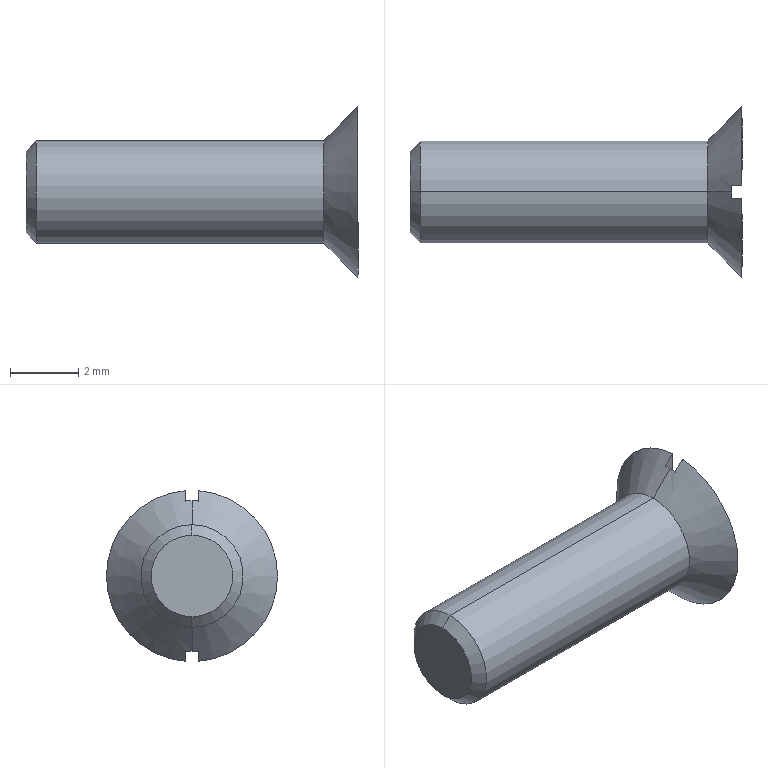Part | SolidWorks | features BaseBody 1 | 1 solid | 12 faces | box 9.7 x 5 x 4.984 mm | volume 73.349 mm3 | plane 6 | cone 4 | cylinder 2 | commonest cylinder face diameters 3 x2
STEP:
#1=CARTESIAN_POINT('',(30.,-10.25,11.75));
#2=VERTEX_POINT('',#1);
#3=CARTESIAN_POINT('',(30.,-10.25,8.75));
#4=VERTEX_POINT('',#3);
#5=CARTESIAN_POINT('',(30.,-10.25,10.25));
#6=DIRECTION('',(-1.,0.,0.));
#7=DIRECTION('',(0.,0.,1.));
#8=AXIS2_PLACEMENT_3D('',#5,#6,#7);
#9=CIRCLE('',#8,1.5);
#10=EDGE_CURVE('',#2,#4,#9,.T.);
#11=ORIENTED_EDGE('',*,*,#10,.T.);
#12=CARTESIAN_POINT('',(21.607,-10.25,8.75));
#13=VERTEX_POINT('',#12);
#14=CARTESIAN_POINT('',(25.803,-10.25,8.75));
#15=DIRECTION('',(-1.,0.,0.));
#16=VECTOR('',#15,1000.);
#17=LINE('',#14,#16);
#18=EDGE_CURVE('',#4,#13,#17,.T.);
#19=ORIENTED_EDGE('',*,*,#18,.T.);
#20=CARTESIAN_POINT('',(21.607,-10.25,11.75));
#21=VERTEX_POINT('',#20);
#22=CARTESIAN_POINT('',(21.607,-10.25,10.25));
#23=DIRECTION('',(1.,0.,0.));
#24=DIRECTION('',(0.,0.,1.));
#25=AXIS2_PLACEMENT_3D('',#22,#23,#24);
#26=CIRCLE('',#25,1.5);
#27=EDGE_CURVE('',#13,#21,#26,.T.);
#28=ORIENTED_EDGE('',*,*,#27,.T.);
#29=CARTESIAN_POINT('',(25.803,-10.25,11.75));
#30=DIRECTION('',(-1.,0.,0.));
#31=VECTOR('',#30,1000.);
#32=LINE('',#29,#31);
#33=EDGE_CURVE('',#2,#21,#32,.T.);
#34=ORIENTED_EDGE('',*,*,#33,.F.);
#35=EDGE_LOOP('',(#11,#19,#28,#34));
#36=FACE_OUTER_BOUND('',#35,.T.);
#37=CARTESIAN_POINT('',(25.803,-10.25,10.25));
#38=DIRECTION('',(-1.,0.,0.));
#39=DIRECTION('',(0.,0.,1.));
#40=AXIS2_PLACEMENT_3D('',#37,#38,#39);
#41=CYLINDRICAL_SURFACE('',#40,1.5);
#42=ADVANCED_FACE('',(#36),#41,.T.);
#43=ORIENTED_EDGE('',*,*,#10,.F.);
#44=CARTESIAN_POINT('',(30.7,-10.25,12.45));
#45=VERTEX_POINT('',#44);
#46=CARTESIAN_POINT('',(31.,-10.25,12.75));
#47=DIRECTION('',(0.7071,0.,0.7071));
#48=VECTOR('',#47,1000.);
#49=LINE('',#46,#48);
#50=EDGE_CURVE('',#2,#45,#49,.T.);
#51=ORIENTED_EDGE('',*,*,#50,.T.);
#52=CARTESIAN_POINT('',(30.7,-10.05,12.441));
#53=VERTEX_POINT('',#52);
#54=CARTESIAN_POINT('',(30.7,-10.25,10.25));
#55=DIRECTION('',(1.,0.,0.));
#56=DIRECTION('',(0.,0.,-1.));
#57=AXIS2_PLACEMENT_3D('',#54,#55,#56);
#58=CIRCLE('',#57,2.2);
#59=EDGE_CURVE('',#53,#45,#58,.T.);
#60=ORIENTED_EDGE('',*,*,#59,.F.);
#61=CARTESIAN_POINT('',(31.,-10.05,12.742));
#62=VERTEX_POINT('',#61);
#63=CARTESIAN_POINT('',(30.7,-10.05,12.441));
#64=CARTESIAN_POINT('',(30.8,-10.05,12.541));
#65=CARTESIAN_POINT('',(30.9,-10.05,12.642));
#66=CARTESIAN_POINT('',(31.,-10.05,12.742));
#67=B_SPLINE_CURVE_WITH_KNOTS('',3,(#63,#64,#65,#66),.UNSPECIFIED.,.F.,.F.,(4,4),(0.,0.000425),.UNSPECIFIED.);
#68=EDGE_CURVE('',#53,#62,#67,.T.);
#69=ORIENTED_EDGE('',*,*,#68,.T.);
#70=CARTESIAN_POINT('',(31.,-10.05,7.758));
#71=VERTEX_POINT('',#70);
#72=CARTESIAN_POINT('',(31.,-10.25,10.25));
#73=DIRECTION('',(-1.,0.,0.));
#74=DIRECTION('',(0.,0.,-1.));
#75=AXIS2_PLACEMENT_3D('',#72,#73,#74);
#76=CIRCLE('',#75,2.5);
#77=EDGE_CURVE('',#62,#71,#76,.T.);
#78=ORIENTED_EDGE('',*,*,#77,.T.);
#79=CARTESIAN_POINT('',(30.7,-10.05,8.059));
#80=VERTEX_POINT('',#79);
#81=CARTESIAN_POINT('',(31.,-10.05,7.758));
#82=CARTESIAN_POINT('',(30.9,-10.05,7.858));
#83=CARTESIAN_POINT('',(30.8,-10.05,7.959));
#84=CARTESIAN_POINT('',(30.7,-10.05,8.059));
#85=B_SPLINE_CURVE_WITH_KNOTS('',3,(#81,#82,#83,#84),.UNSPECIFIED.,.F.,.F.,(4,4),(0.,0.000425),.UNSPECIFIED.);
#86=EDGE_CURVE('',#71,#80,#85,.T.);
#87=ORIENTED_EDGE('',*,*,#86,.T.);
#88=CARTESIAN_POINT('',(30.7,-10.25,8.05));
#89=VERTEX_POINT('',#88);
#90=CARTESIAN_POINT('',(30.7,-10.25,10.25));
#91=DIRECTION('',(1.,0.,0.));
#92=DIRECTION('',(0.,0.,-1.));
#93=AXIS2_PLACEMENT_3D('',#90,#91,#92);
#94=CIRCLE('',#93,2.2);
#95=EDGE_CURVE('',#89,#80,#94,.T.);
#96=ORIENTED_EDGE('',*,*,#95,.F.);
#97=CARTESIAN_POINT('',(31.,-10.25,7.75));
#98=DIRECTION('',(0.7071,0.,-0.7071));
#99=VECTOR('',#98,1000.);
#100=LINE('',#97,#99);
#101=EDGE_CURVE('',#4,#89,#100,.T.);
#102=ORIENTED_EDGE('',*,*,#101,.F.);
#103=EDGE_LOOP('',(#43,#51,#60,#69,#78,#87,#96,#102));
#104=FACE_OUTER_BOUND('',#103,.T.);
#105=CARTESIAN_POINT('',(31.,-10.25,10.25));
#106=DIRECTION('',(1.,0.,0.));
#107=DIRECTION('',(0.,0.,-1.));
#108=AXIS2_PLACEMENT_3D('',#105,#106,#107);
#109=CONICAL_SURFACE('',#108,2.5,0.7854);
#110=ADVANCED_FACE('',(#104),#109,.T.);
#111=CARTESIAN_POINT('',(21.3,-10.25,9.057));
#112=VERTEX_POINT('',#111);
#113=CARTESIAN_POINT('',(21.3,-10.25,11.443));
#114=VERTEX_POINT('',#113);
#115=CARTESIAN_POINT('',(21.3,-10.25,10.25));
#116=DIRECTION('',(1.,0.,0.));
#117=DIRECTION('',(0.,0.,-1.));
#118=AXIS2_PLACEMENT_3D('',#115,#116,#117);
#119=CIRCLE('',#118,1.193);
#120=EDGE_CURVE('',#112,#114,#119,.T.);
#121=ORIENTED_EDGE('',*,*,#120,.T.);
#122=CARTESIAN_POINT('',(21.607,-10.25,11.75));
#123=DIRECTION('',(0.7071,0.,0.7071));
#124=VECTOR('',#123,1000.);
#125=LINE('',#122,#124);
#126=EDGE_CURVE('',#114,#21,#125,.T.);
#127=ORIENTED_EDGE('',*,*,#126,.T.);
#128=ORIENTED_EDGE('',*,*,#27,.F.);
#129=CARTESIAN_POINT('',(21.607,-10.25,8.75));
#130=DIRECTION('',(0.7071,0.,-0.7071));
#131=VECTOR('',#130,1000.);
#132=LINE('',#129,#131);
#133=EDGE_CURVE('',#112,#13,#132,.T.);
#134=ORIENTED_EDGE('',*,*,#133,.F.);
#135=EDGE_LOOP('',(#121,#127,#128,#134));
#136=FACE_OUTER_BOUND('',#135,.T.);
#137=CARTESIAN_POINT('',(21.607,-10.25,10.25));
#138=DIRECTION('',(1.,0.,0.));
#139=DIRECTION('',(0.,0.,-1.));
#140=AXIS2_PLACEMENT_3D('',#137,#138,#139);
#141=CONICAL_SURFACE('',#140,1.5,0.7854);
#142=ADVANCED_FACE('',(#136),#141,.T.);
#143=CARTESIAN_POINT('',(30.7,-10.45,12.441));
#144=VERTEX_POINT('',#143);
#145=CARTESIAN_POINT('',(30.7,-10.45,8.059));
#146=VERTEX_POINT('',#145);
#147=CARTESIAN_POINT('',(30.7,-10.45,12.75));
#148=DIRECTION('',(0.,0.,-1.));
#149=VECTOR('',#148,1000.);
#150=LINE('',#147,#149);
#151=EDGE_CURVE('',#144,#146,#150,.T.);
#152=ORIENTED_EDGE('',*,*,#151,.T.);
#153=CARTESIAN_POINT('',(30.7,-10.25,10.25));
#154=DIRECTION('',(1.,0.,0.));
#155=DIRECTION('',(0.,0.,-1.));
#156=AXIS2_PLACEMENT_3D('',#153,#154,#155);
#157=CIRCLE('',#156,2.2);
#158=EDGE_CURVE('',#146,#89,#157,.T.);
#159=ORIENTED_EDGE('',*,*,#158,.T.);
#160=ORIENTED_EDGE('',*,*,#95,.T.);
#161=CARTESIAN_POINT('',(30.7,-10.05,7.75));
#162=DIRECTION('',(0.,0.,1.));
#163=VECTOR('',#162,1000.);
#164=LINE('',#161,#163);
#165=EDGE_CURVE('',#80,#53,#164,.T.);
#166=ORIENTED_EDGE('',*,*,#165,.T.);
#167=ORIENTED_EDGE('',*,*,#59,.T.);
#168=CARTESIAN_POINT('',(30.7,-10.25,10.25));
#169=DIRECTION('',(1.,0.,0.));
#170=DIRECTION('',(0.,0.,-1.));
#171=AXIS2_PLACEMENT_3D('',#168,#169,#170);
#172=CIRCLE('',#171,2.2);
#173=EDGE_CURVE('',#45,#144,#172,.T.);
#174=ORIENTED_EDGE('',*,*,#173,.T.);
#175=EDGE_LOOP('',(#152,#159,#160,#166,#167,#174));
#176=FACE_OUTER_BOUND('',#175,.T.);
#177=CARTESIAN_POINT('',(30.7,-10.25,10.25));
#178=DIRECTION('',(1.,0.,0.));
#179=DIRECTION('',(0.,1.,0.));
#180=AXIS2_PLACEMENT_3D('',#177,#178,#179);
#181=PLANE('',#180);
#182=ADVANCED_FACE('',(#176),#181,.T.);
#183=CARTESIAN_POINT('',(31.,-10.45,7.758));
#184=VERTEX_POINT('',#183);
#185=CARTESIAN_POINT('',(31.,-10.45,12.742));
#186=VERTEX_POINT('',#185);
#187=CARTESIAN_POINT('',(31.,-10.45,10.25));
#188=DIRECTION('',(0.,0.,1.));
#189=VECTOR('',#188,1000.);
#190=LINE('',#187,#189);
#191=EDGE_CURVE('',#184,#186,#190,.T.);
#192=ORIENTED_EDGE('',*,*,#191,.F.);
#193=CARTESIAN_POINT('',(30.7,-10.45,8.059));
#194=CARTESIAN_POINT('',(30.8,-10.45,7.959));
#195=CARTESIAN_POINT('',(30.9,-10.45,7.858));
#196=CARTESIAN_POINT('',(31.,-10.45,7.758));
#197=B_SPLINE_CURVE_WITH_KNOTS('',3,(#193,#194,#195,#196),.UNSPECIFIED.,.F.,.F.,(4,4),(0.,0.000425),.UNSPECIFIED.);
#198=EDGE_CURVE('',#146,#184,#197,.T.);
#199=ORIENTED_EDGE('',*,*,#198,.F.);
#200=ORIENTED_EDGE('',*,*,#151,.F.);
#201=CARTESIAN_POINT('',(31.,-10.45,12.742));
#202=CARTESIAN_POINT('',(30.9,-10.45,12.642));
#203=CARTESIAN_POINT('',(30.8,-10.45,12.541));
#204=CARTESIAN_POINT('',(30.7,-10.45,12.441));
#205=B_SPLINE_CURVE_WITH_KNOTS('',3,(#201,#202,#203,#204),.UNSPECIFIED.,.F.,.F.,(4,4),(0.,0.000425),.UNSPECIFIED.);
#206=EDGE_CURVE('',#186,#144,#205,.T.);
#207=ORIENTED_EDGE('',*,*,#206,.F.);
#208=EDGE_LOOP('',(#192,#199,#200,#207));
#209=FACE_OUTER_BOUND('',#208,.T.);
#210=CARTESIAN_POINT('',(31.,-10.45,12.75));
#211=DIRECTION('',(0.,-1.,0.));
#212=DIRECTION('',(0.,0.,-1.));
#213=AXIS2_PLACEMENT_3D('',#210,#211,#212);
#214=PLANE('',#213);
#215=ADVANCED_FACE('',(#209),#214,.F.);
#216=ORIENTED_EDGE('',*,*,#165,.F.);
#217=ORIENTED_EDGE('',*,*,#86,.F.);
#218=CARTESIAN_POINT('',(31.,-10.05,10.25));
#219=DIRECTION('',(0.,0.,-1.));
#220=VECTOR('',#219,1000.);
#221=LINE('',#218,#220);
#222=EDGE_CURVE('',#62,#71,#221,.T.);
#223=ORIENTED_EDGE('',*,*,#222,.F.);
#224=ORIENTED_EDGE('',*,*,#68,.F.);
#225=EDGE_LOOP('',(#216,#217,#223,#224));
#226=FACE_OUTER_BOUND('',#225,.T.);
#227=CARTESIAN_POINT('',(31.,-10.05,7.75));
#228=DIRECTION('',(0.,1.,0.));
#229=DIRECTION('',(1.,0.,0.));
#230=AXIS2_PLACEMENT_3D('',#227,#228,#229);
#231=PLANE('',#230);
#232=ADVANCED_FACE('',(#226),#231,.F.);
#233=ORIENTED_EDGE('',*,*,#120,.F.);
#234=CARTESIAN_POINT('',(21.3,-10.25,10.25));
#235=DIRECTION('',(1.,0.,0.));
#236=DIRECTION('',(0.,0.,-1.));
#237=AXIS2_PLACEMENT_3D('',#234,#235,#236);
#238=CIRCLE('',#237,1.193);
#239=EDGE_CURVE('',#114,#112,#238,.T.);
#240=ORIENTED_EDGE('',*,*,#239,.F.);
#241=EDGE_LOOP('',(#233,#240));
#242=FACE_OUTER_BOUND('',#241,.T.);
#243=CARTESIAN_POINT('',(21.3,-9.653,10.25));
#244=DIRECTION('',(-1.,0.,0.));
#245=DIRECTION('',(0.,0.,1.));
#246=AXIS2_PLACEMENT_3D('',#243,#244,#245);
#247=PLANE('',#246);
#248=ADVANCED_FACE('',(#242),#247,.T.);
#249=CARTESIAN_POINT('',(31.,-10.25,10.25));
#250=DIRECTION('',(-1.,0.,0.));
#251=DIRECTION('',(0.,0.,-1.));
#252=AXIS2_PLACEMENT_3D('',#249,#250,#251);
#253=CIRCLE('',#252,2.5);
#254=EDGE_CURVE('',#184,#186,#253,.T.);
#255=ORIENTED_EDGE('',*,*,#254,.F.);
#256=ORIENTED_EDGE('',*,*,#191,.T.);
#257=EDGE_LOOP('',(#255,#256));
#258=FACE_OUTER_BOUND('',#257,.T.);
#259=CARTESIAN_POINT('',(31.,-9.,10.25));
#260=DIRECTION('',(1.,0.,0.));
#261=DIRECTION('',(0.,1.,0.));
#262=AXIS2_PLACEMENT_3D('',#259,#260,#261);
#263=PLANE('',#262);
#264=ADVANCED_FACE('',(#258),#263,.T.);
#265=ORIENTED_EDGE('',*,*,#222,.T.);
#266=ORIENTED_EDGE('',*,*,#77,.F.);
#267=EDGE_LOOP('',(#265,#266));
#268=FACE_OUTER_BOUND('',#267,.T.);
#269=CARTESIAN_POINT('',(31.,-9.,10.25));
#270=DIRECTION('',(1.,0.,0.));
#271=DIRECTION('',(0.,1.,0.));
#272=AXIS2_PLACEMENT_3D('',#269,#270,#271);
#273=PLANE('',#272);
#274=ADVANCED_FACE('',(#268),#273,.T.);
#275=ORIENTED_EDGE('',*,*,#126,.F.);
#276=ORIENTED_EDGE('',*,*,#239,.T.);
#277=ORIENTED_EDGE('',*,*,#133,.T.);
#278=CARTESIAN_POINT('',(21.607,-10.25,10.25));
#279=DIRECTION('',(1.,0.,0.));
#280=DIRECTION('',(0.,0.,1.));
#281=AXIS2_PLACEMENT_3D('',#278,#279,#280);
#282=CIRCLE('',#281,1.5);
#283=EDGE_CURVE('',#21,#13,#282,.T.);
#284=ORIENTED_EDGE('',*,*,#283,.F.);
#285=EDGE_LOOP('',(#275,#276,#277,#284));
#286=FACE_OUTER_BOUND('',#285,.T.);
#287=CARTESIAN_POINT('',(21.607,-10.25,10.25));
#288=DIRECTION('',(1.,0.,0.));
#289=DIRECTION('',(0.,0.,-1.));
#290=AXIS2_PLACEMENT_3D('',#287,#288,#289);
#291=CONICAL_SURFACE('',#290,1.5,0.7854);
#292=ADVANCED_FACE('',(#286),#291,.T.);
#293=ORIENTED_EDGE('',*,*,#50,.F.);
#294=CARTESIAN_POINT('',(30.,-10.25,10.25));
#295=DIRECTION('',(-1.,0.,0.));
#296=DIRECTION('',(0.,0.,1.));
#297=AXIS2_PLACEMENT_3D('',#294,#295,#296);
#298=CIRCLE('',#297,1.5);
#299=EDGE_CURVE('',#4,#2,#298,.T.);
#300=ORIENTED_EDGE('',*,*,#299,.F.);
#301=ORIENTED_EDGE('',*,*,#101,.T.);
#302=ORIENTED_EDGE('',*,*,#158,.F.);
#303=ORIENTED_EDGE('',*,*,#198,.T.);
#304=ORIENTED_EDGE('',*,*,#254,.T.);
#305=ORIENTED_EDGE('',*,*,#206,.T.);
#306=ORIENTED_EDGE('',*,*,#173,.F.);
#307=EDGE_LOOP('',(#293,#300,#301,#302,#303,#304,#305,#306));
#308=FACE_OUTER_BOUND('',#307,.T.);
#309=CARTESIAN_POINT('',(31.,-10.25,10.25));
#310=DIRECTION('',(1.,0.,0.));
#311=DIRECTION('',(0.,0.,-1.));
#312=AXIS2_PLACEMENT_3D('',#309,#310,#311);
#313=CONICAL_SURFACE('',#312,2.5,0.7854);
#314=ADVANCED_FACE('',(#308),#313,.T.);
#315=ORIENTED_EDGE('',*,*,#18,.F.);
#316=ORIENTED_EDGE('',*,*,#299,.T.);
#317=ORIENTED_EDGE('',*,*,#33,.T.);
#318=ORIENTED_EDGE('',*,*,#283,.T.);
#319=EDGE_LOOP('',(#315,#316,#317,#318));
#320=FACE_OUTER_BOUND('',#319,.T.);
#321=CARTESIAN_POINT('',(25.803,-10.25,10.25));
#322=DIRECTION('',(-1.,0.,0.));
#323=DIRECTION('',(0.,0.,1.));
#324=AXIS2_PLACEMENT_3D('',#321,#322,#323);
#325=CYLINDRICAL_SURFACE('',#324,1.5);
#326=ADVANCED_FACE('',(#320),#325,.T.);
#327=CLOSED_SHELL('',(#42,#110,#142,#182,#215,#232,#248,#264,#274,#292,#314,#326));
#328=MANIFOLD_SOLID_BREP('',#327);
#329=CARTESIAN_POINT('',(0.,0.,0.));
#330=DIRECTION('',(0.,0.,1.));
#331=DIRECTION('',(1.,0.,0.));
#332=AXIS2_PLACEMENT_3D('',#329,#330,#331);
#333=(LENGTH_UNIT()NAMED_UNIT(*)SI_UNIT(.MILLI.,.METRE.));
#334=UNCERTAINTY_MEASURE_WITH_UNIT(LENGTH_MEASURE(0.00001),#333,'','');
#335=(NAMED_UNIT(*)PLANE_ANGLE_UNIT()SI_UNIT($,.RADIAN.));
#336=(NAMED_UNIT(*)SI_UNIT($,.STERADIAN.)SOLID_ANGLE_UNIT());
#337=(GEOMETRIC_REPRESENTATION_CONTEXT(3)GLOBAL_UNCERTAINTY_ASSIGNED_CONTEXT((#334))GLOBAL_UNIT_ASSIGNED_CONTEXT((#333,#335,#336))REPRESENTATION_CONTEXT('',''));
#338=ADVANCED_BREP_SHAPE_REPRESENTATION('',(#328,#332),#337);